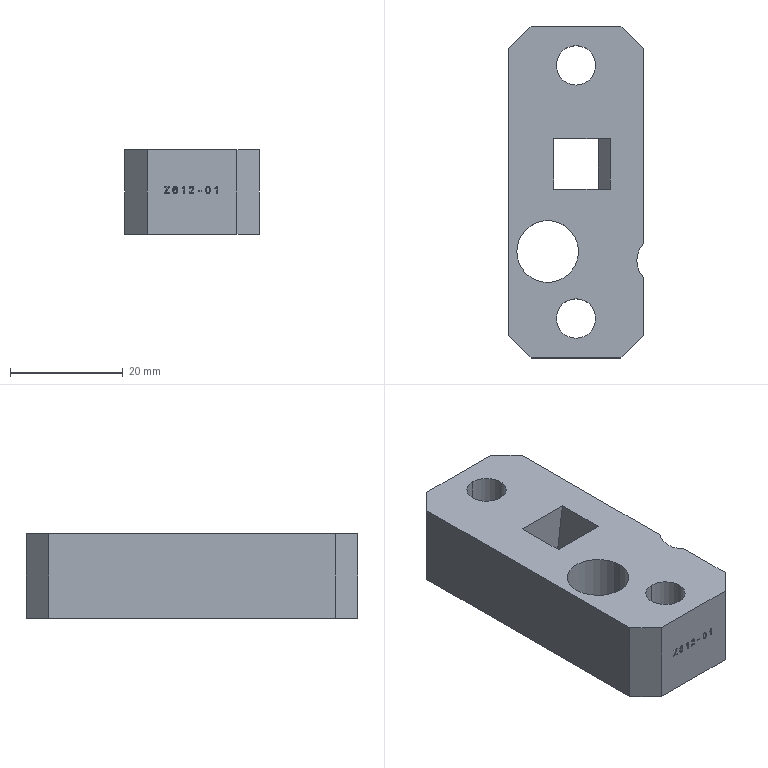Part | Creo | 1 solid | 141 faces | box 24 x 59 x 15 mm | volume 15950 mm3 | other 77 | plane 51 | cylinder 13 | commonest cylinder face diameters 11 x6 7 x4 1.137 x1 9 x1 17.925 x1